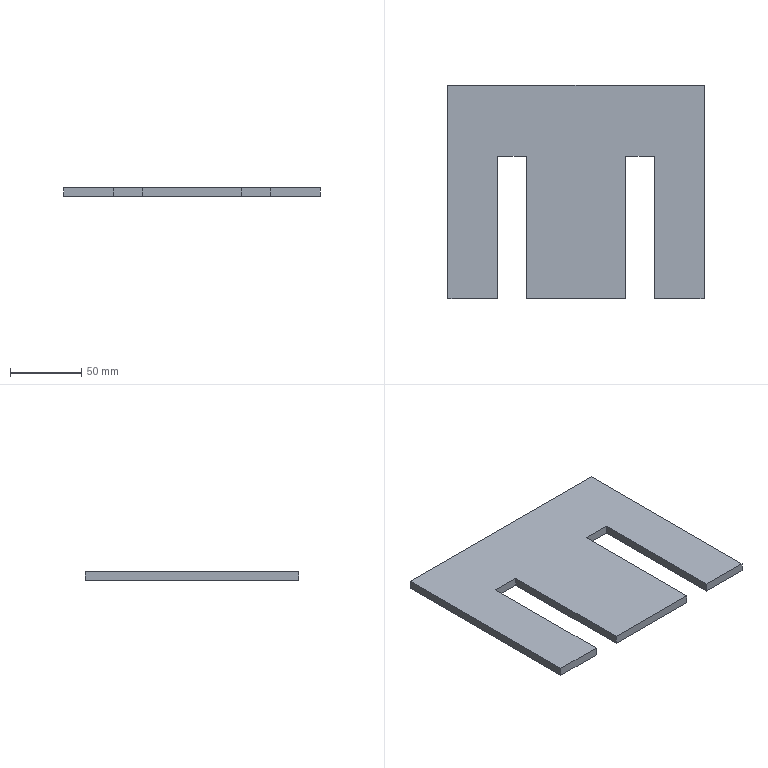Part | SolidWorks | features Extrusion 1, ICE 1, MirrorPattern 1 | 1 solid | 14 faces | box 180 x 150 x 6 mm | volume 138000 mm3 | plane 14
STEP:
#1=CARTESIAN_POINT('',(55.,-75.,0.));
#2=VERTEX_POINT('',#1);
#3=CARTESIAN_POINT('',(55.,-75.,6.));
#4=VERTEX_POINT('',#3);
#5=CARTESIAN_POINT('',(55.,-75.,-0.001));
#6=DIRECTION('',(0.,0.,1.));
#7=VECTOR('',#6,1000.);
#8=LINE('',#5,#7);
#9=EDGE_CURVE('',#2,#4,#8,.T.);
#10=ORIENTED_EDGE('',*,*,#9,.F.);
#11=CARTESIAN_POINT('',(90.,-75.,0.));
#12=VERTEX_POINT('',#11);
#13=CARTESIAN_POINT('',(-90.,-75.,0.));
#14=DIRECTION('',(1.,0.,0.));
#15=VECTOR('',#14,1000.);
#16=LINE('',#13,#15);
#17=EDGE_CURVE('',#2,#12,#16,.T.);
#18=ORIENTED_EDGE('',*,*,#17,.T.);
#19=CARTESIAN_POINT('',(90.,-75.,6.));
#20=VERTEX_POINT('',#19);
#21=CARTESIAN_POINT('',(90.,-75.,6.));
#22=DIRECTION('',(0.,0.,-1.));
#23=VECTOR('',#22,1000.);
#24=LINE('',#21,#23);
#25=EDGE_CURVE('',#20,#12,#24,.T.);
#26=ORIENTED_EDGE('',*,*,#25,.F.);
#27=CARTESIAN_POINT('',(-90.,-75.,6.));
#28=DIRECTION('',(1.,0.,0.));
#29=VECTOR('',#28,1000.);
#30=LINE('',#27,#29);
#31=EDGE_CURVE('',#4,#20,#30,.T.);
#32=ORIENTED_EDGE('',*,*,#31,.F.);
#33=EDGE_LOOP('',(#10,#18,#26,#32));
#34=FACE_OUTER_BOUND('',#33,.T.);
#35=CARTESIAN_POINT('',(-90.,-75.,6.));
#36=DIRECTION('',(0.,1.,0.));
#37=DIRECTION('',(0.,0.,1.));
#38=AXIS2_PLACEMENT_3D('',#35,#36,#37);
#39=PLANE('',#38);
#40=ADVANCED_FACE('',(#34),#39,.F.);
#41=CARTESIAN_POINT('',(35.,-75.,0.));
#42=VERTEX_POINT('',#41);
#43=CARTESIAN_POINT('',(35.,-75.,6.));
#44=VERTEX_POINT('',#43);
#45=CARTESIAN_POINT('',(35.,-75.,-0.001));
#46=DIRECTION('',(0.,0.,1.));
#47=VECTOR('',#46,1000.);
#48=LINE('',#45,#47);
#49=EDGE_CURVE('',#42,#44,#48,.T.);
#50=ORIENTED_EDGE('',*,*,#49,.T.);
#51=CARTESIAN_POINT('',(-35.,-75.,6.));
#52=VERTEX_POINT('',#51);
#53=CARTESIAN_POINT('',(-90.,-75.,6.));
#54=DIRECTION('',(1.,0.,0.));
#55=VECTOR('',#54,1000.);
#56=LINE('',#53,#55);
#57=EDGE_CURVE('',#52,#44,#56,.T.);
#58=ORIENTED_EDGE('',*,*,#57,.F.);
#59=CARTESIAN_POINT('',(-35.,-75.,0.));
#60=VERTEX_POINT('',#59);
#61=CARTESIAN_POINT('',(-35.,-75.,-0.001));
#62=DIRECTION('',(0.,0.,1.));
#63=VECTOR('',#62,1000.);
#64=LINE('',#61,#63);
#65=EDGE_CURVE('',#60,#52,#64,.T.);
#66=ORIENTED_EDGE('',*,*,#65,.F.);
#67=CARTESIAN_POINT('',(-90.,-75.,0.));
#68=DIRECTION('',(1.,0.,0.));
#69=VECTOR('',#68,1000.);
#70=LINE('',#67,#69);
#71=EDGE_CURVE('',#60,#42,#70,.T.);
#72=ORIENTED_EDGE('',*,*,#71,.T.);
#73=EDGE_LOOP('',(#50,#58,#66,#72));
#74=FACE_OUTER_BOUND('',#73,.T.);
#75=CARTESIAN_POINT('',(-90.,-75.,6.));
#76=DIRECTION('',(0.,1.,0.));
#77=DIRECTION('',(0.,0.,1.));
#78=AXIS2_PLACEMENT_3D('',#75,#76,#77);
#79=PLANE('',#78);
#80=ADVANCED_FACE('',(#74),#79,.F.);
#81=CARTESIAN_POINT('',(55.,25.,6.));
#82=VERTEX_POINT('',#81);
#83=CARTESIAN_POINT('',(55.,-75.,6.));
#84=DIRECTION('',(0.,-1.,0.));
#85=VECTOR('',#84,1000.);
#86=LINE('',#83,#85);
#87=EDGE_CURVE('',#82,#4,#86,.T.);
#88=ORIENTED_EDGE('',*,*,#87,.T.);
#89=ORIENTED_EDGE('',*,*,#31,.T.);
#90=CARTESIAN_POINT('',(90.,75.,6.));
#91=VERTEX_POINT('',#90);
#92=CARTESIAN_POINT('',(90.,-75.,6.));
#93=DIRECTION('',(0.,1.,0.));
#94=VECTOR('',#93,1000.);
#95=LINE('',#92,#94);
#96=EDGE_CURVE('',#20,#91,#95,.T.);
#97=ORIENTED_EDGE('',*,*,#96,.T.);
#98=CARTESIAN_POINT('',(-90.,75.,6.));
#99=VERTEX_POINT('',#98);
#100=CARTESIAN_POINT('',(-90.,75.,6.));
#101=DIRECTION('',(-1.,0.,0.));
#102=VECTOR('',#101,1000.);
#103=LINE('',#100,#102);
#104=EDGE_CURVE('',#91,#99,#103,.T.);
#105=ORIENTED_EDGE('',*,*,#104,.T.);
#106=CARTESIAN_POINT('',(-90.,-75.,6.));
#107=VERTEX_POINT('',#106);
#108=CARTESIAN_POINT('',(-90.,-75.,6.));
#109=DIRECTION('',(0.,-1.,0.));
#110=VECTOR('',#109,1000.);
#111=LINE('',#108,#110);
#112=EDGE_CURVE('',#99,#107,#111,.T.);
#113=ORIENTED_EDGE('',*,*,#112,.T.);
#114=CARTESIAN_POINT('',(-55.,-75.,6.));
#115=VERTEX_POINT('',#114);
#116=CARTESIAN_POINT('',(-90.,-75.,6.));
#117=DIRECTION('',(1.,0.,0.));
#118=VECTOR('',#117,1000.);
#119=LINE('',#116,#118);
#120=EDGE_CURVE('',#107,#115,#119,.T.);
#121=ORIENTED_EDGE('',*,*,#120,.T.);
#122=CARTESIAN_POINT('',(-55.,25.,6.));
#123=VERTEX_POINT('',#122);
#124=CARTESIAN_POINT('',(-55.,-75.,6.));
#125=DIRECTION('',(0.,-1.,0.));
#126=VECTOR('',#125,1000.);
#127=LINE('',#124,#126);
#128=EDGE_CURVE('',#123,#115,#127,.T.);
#129=ORIENTED_EDGE('',*,*,#128,.F.);
#130=CARTESIAN_POINT('',(-35.,25.,6.));
#131=VERTEX_POINT('',#130);
#132=CARTESIAN_POINT('',(-55.,25.,6.));
#133=DIRECTION('',(-1.,0.,0.));
#134=VECTOR('',#133,1000.);
#135=LINE('',#132,#134);
#136=EDGE_CURVE('',#131,#123,#135,.T.);
#137=ORIENTED_EDGE('',*,*,#136,.F.);
#138=CARTESIAN_POINT('',(-35.,-75.,6.));
#139=DIRECTION('',(0.,1.,0.));
#140=VECTOR('',#139,1000.);
#141=LINE('',#138,#140);
#142=EDGE_CURVE('',#52,#131,#141,.T.);
#143=ORIENTED_EDGE('',*,*,#142,.F.);
#144=ORIENTED_EDGE('',*,*,#57,.T.);
#145=CARTESIAN_POINT('',(35.,25.,6.));
#146=VERTEX_POINT('',#145);
#147=CARTESIAN_POINT('',(35.,-75.,6.));
#148=DIRECTION('',(0.,1.,0.));
#149=VECTOR('',#148,1000.);
#150=LINE('',#147,#149);
#151=EDGE_CURVE('',#44,#146,#150,.T.);
#152=ORIENTED_EDGE('',*,*,#151,.T.);
#153=CARTESIAN_POINT('',(55.,25.,6.));
#154=DIRECTION('',(1.,0.,0.));
#155=VECTOR('',#154,1000.);
#156=LINE('',#153,#155);
#157=EDGE_CURVE('',#146,#82,#156,.T.);
#158=ORIENTED_EDGE('',*,*,#157,.T.);
#159=EDGE_LOOP('',(#88,#89,#97,#105,#113,#121,#129,#137,#143,#144,#152,#158));
#160=FACE_OUTER_BOUND('',#159,.T.);
#161=CARTESIAN_POINT('',(0.,0.,6.));
#162=DIRECTION('',(0.,0.,-1.));
#163=DIRECTION('',(-1.,0.,0.));
#164=AXIS2_PLACEMENT_3D('',#161,#162,#163);
#165=PLANE('',#164);
#166=ADVANCED_FACE('',(#160),#165,.F.);
#167=ORIENTED_EDGE('',*,*,#17,.F.);
#168=CARTESIAN_POINT('',(55.,25.,0.));
#169=VERTEX_POINT('',#168);
#170=CARTESIAN_POINT('',(55.,-75.,0.));
#171=DIRECTION('',(0.,-1.,0.));
#172=VECTOR('',#171,1000.);
#173=LINE('',#170,#172);
#174=EDGE_CURVE('',#169,#2,#173,.T.);
#175=ORIENTED_EDGE('',*,*,#174,.F.);
#176=CARTESIAN_POINT('',(35.,25.,0.));
#177=VERTEX_POINT('',#176);
#178=CARTESIAN_POINT('',(55.,25.,0.));
#179=DIRECTION('',(1.,0.,0.));
#180=VECTOR('',#179,1000.);
#181=LINE('',#178,#180);
#182=EDGE_CURVE('',#177,#169,#181,.T.);
#183=ORIENTED_EDGE('',*,*,#182,.F.);
#184=CARTESIAN_POINT('',(35.,-75.,0.));
#185=DIRECTION('',(0.,1.,0.));
#186=VECTOR('',#185,1000.);
#187=LINE('',#184,#186);
#188=EDGE_CURVE('',#42,#177,#187,.T.);
#189=ORIENTED_EDGE('',*,*,#188,.F.);
#190=ORIENTED_EDGE('',*,*,#71,.F.);
#191=CARTESIAN_POINT('',(-35.,25.,0.));
#192=VERTEX_POINT('',#191);
#193=CARTESIAN_POINT('',(-35.,-75.,0.));
#194=DIRECTION('',(0.,1.,0.));
#195=VECTOR('',#194,1000.);
#196=LINE('',#193,#195);
#197=EDGE_CURVE('',#60,#192,#196,.T.);
#198=ORIENTED_EDGE('',*,*,#197,.T.);
#199=CARTESIAN_POINT('',(-55.,25.,0.));
#200=VERTEX_POINT('',#199);
#201=CARTESIAN_POINT('',(-55.,25.,0.));
#202=DIRECTION('',(-1.,0.,0.));
#203=VECTOR('',#202,1000.);
#204=LINE('',#201,#203);
#205=EDGE_CURVE('',#192,#200,#204,.T.);
#206=ORIENTED_EDGE('',*,*,#205,.T.);
#207=CARTESIAN_POINT('',(-55.,-75.,0.));
#208=VERTEX_POINT('',#207);
#209=CARTESIAN_POINT('',(-55.,-75.,0.));
#210=DIRECTION('',(0.,-1.,0.));
#211=VECTOR('',#210,1000.);
#212=LINE('',#209,#211);
#213=EDGE_CURVE('',#200,#208,#212,.T.);
#214=ORIENTED_EDGE('',*,*,#213,.T.);
#215=CARTESIAN_POINT('',(-90.,-75.,0.));
#216=VERTEX_POINT('',#215);
#217=CARTESIAN_POINT('',(-90.,-75.,0.));
#218=DIRECTION('',(1.,0.,0.));
#219=VECTOR('',#218,1000.);
#220=LINE('',#217,#219);
#221=EDGE_CURVE('',#216,#208,#220,.T.);
#222=ORIENTED_EDGE('',*,*,#221,.F.);
#223=CARTESIAN_POINT('',(-90.,75.,0.));
#224=VERTEX_POINT('',#223);
#225=CARTESIAN_POINT('',(-90.,-75.,0.));
#226=DIRECTION('',(0.,-1.,0.));
#227=VECTOR('',#226,1000.);
#228=LINE('',#225,#227);
#229=EDGE_CURVE('',#224,#216,#228,.T.);
#230=ORIENTED_EDGE('',*,*,#229,.F.);
#231=CARTESIAN_POINT('',(90.,75.,0.));
#232=VERTEX_POINT('',#231);
#233=CARTESIAN_POINT('',(-90.,75.,0.));
#234=DIRECTION('',(-1.,0.,0.));
#235=VECTOR('',#234,1000.);
#236=LINE('',#233,#235);
#237=EDGE_CURVE('',#232,#224,#236,.T.);
#238=ORIENTED_EDGE('',*,*,#237,.F.);
#239=CARTESIAN_POINT('',(90.,-75.,0.));
#240=DIRECTION('',(0.,1.,0.));
#241=VECTOR('',#240,1000.);
#242=LINE('',#239,#241);
#243=EDGE_CURVE('',#12,#232,#242,.T.);
#244=ORIENTED_EDGE('',*,*,#243,.F.);
#245=EDGE_LOOP('',(#167,#175,#183,#189,#190,#198,#206,#214,#222,#230,#238,#244));
#246=FACE_OUTER_BOUND('',#245,.T.);
#247=CARTESIAN_POINT('',(0.,0.,0.));
#248=DIRECTION('',(0.,0.,-1.));
#249=DIRECTION('',(-1.,0.,0.));
#250=AXIS2_PLACEMENT_3D('',#247,#248,#249);
#251=PLANE('',#250);
#252=ADVANCED_FACE('',(#246),#251,.T.);
#253=ORIENTED_EDGE('',*,*,#221,.T.);
#254=CARTESIAN_POINT('',(-55.,-75.,-0.001));
#255=DIRECTION('',(0.,0.,1.));
#256=VECTOR('',#255,1000.);
#257=LINE('',#254,#256);
#258=EDGE_CURVE('',#208,#115,#257,.T.);
#259=ORIENTED_EDGE('',*,*,#258,.T.);
#260=ORIENTED_EDGE('',*,*,#120,.F.);
#261=CARTESIAN_POINT('',(-90.,-75.,6.));
#262=DIRECTION('',(0.,0.,-1.));
#263=VECTOR('',#262,1000.);
#264=LINE('',#261,#263);
#265=EDGE_CURVE('',#107,#216,#264,.T.);
#266=ORIENTED_EDGE('',*,*,#265,.T.);
#267=EDGE_LOOP('',(#253,#259,#260,#266));
#268=FACE_OUTER_BOUND('',#267,.T.);
#269=CARTESIAN_POINT('',(-90.,-75.,6.));
#270=DIRECTION('',(0.,1.,0.));
#271=DIRECTION('',(0.,0.,1.));
#272=AXIS2_PLACEMENT_3D('',#269,#270,#271);
#273=PLANE('',#272);
#274=ADVANCED_FACE('',(#268),#273,.F.);
#275=ORIENTED_EDGE('',*,*,#243,.T.);
#276=CARTESIAN_POINT('',(90.,75.,6.));
#277=DIRECTION('',(0.,0.,-1.));
#278=VECTOR('',#277,1000.);
#279=LINE('',#276,#278);
#280=EDGE_CURVE('',#91,#232,#279,.T.);
#281=ORIENTED_EDGE('',*,*,#280,.F.);
#282=ORIENTED_EDGE('',*,*,#96,.F.);
#283=ORIENTED_EDGE('',*,*,#25,.T.);
#284=EDGE_LOOP('',(#275,#281,#282,#283));
#285=FACE_OUTER_BOUND('',#284,.T.);
#286=CARTESIAN_POINT('',(90.,-75.,6.));
#287=DIRECTION('',(-1.,0.,0.));
#288=DIRECTION('',(0.,0.,1.));
#289=AXIS2_PLACEMENT_3D('',#286,#287,#288);
#290=PLANE('',#289);
#291=ADVANCED_FACE('',(#285),#290,.F.);
#292=ORIENTED_EDGE('',*,*,#237,.T.);
#293=CARTESIAN_POINT('',(-90.,75.,6.));
#294=DIRECTION('',(0.,0.,-1.));
#295=VECTOR('',#294,1000.);
#296=LINE('',#293,#295);
#297=EDGE_CURVE('',#99,#224,#296,.T.);
#298=ORIENTED_EDGE('',*,*,#297,.F.);
#299=ORIENTED_EDGE('',*,*,#104,.F.);
#300=ORIENTED_EDGE('',*,*,#280,.T.);
#301=EDGE_LOOP('',(#292,#298,#299,#300));
#302=FACE_OUTER_BOUND('',#301,.T.);
#303=CARTESIAN_POINT('',(-90.,75.,6.));
#304=DIRECTION('',(0.,-1.,0.));
#305=DIRECTION('',(0.,0.,-1.));
#306=AXIS2_PLACEMENT_3D('',#303,#304,#305);
#307=PLANE('',#306);
#308=ADVANCED_FACE('',(#302),#307,.F.);
#309=ORIENTED_EDGE('',*,*,#229,.T.);
#310=ORIENTED_EDGE('',*,*,#265,.F.);
#311=ORIENTED_EDGE('',*,*,#112,.F.);
#312=ORIENTED_EDGE('',*,*,#297,.T.);
#313=EDGE_LOOP('',(#309,#310,#311,#312));
#314=FACE_OUTER_BOUND('',#313,.T.);
#315=CARTESIAN_POINT('',(-90.,-75.,6.));
#316=DIRECTION('',(1.,0.,0.));
#317=DIRECTION('',(0.,0.,-1.));
#318=AXIS2_PLACEMENT_3D('',#315,#316,#317);
#319=PLANE('',#318);
#320=ADVANCED_FACE('',(#314),#319,.F.);
#321=CARTESIAN_POINT('',(-55.,25.,-0.001));
#322=DIRECTION('',(0.,0.,1.));
#323=VECTOR('',#322,1000.);
#324=LINE('',#321,#323);
#325=EDGE_CURVE('',#200,#123,#324,.T.);
#326=ORIENTED_EDGE('',*,*,#325,.T.);
#327=ORIENTED_EDGE('',*,*,#128,.T.);
#328=ORIENTED_EDGE('',*,*,#258,.F.);
#329=ORIENTED_EDGE('',*,*,#213,.F.);
#330=EDGE_LOOP('',(#326,#327,#328,#329));
#331=FACE_OUTER_BOUND('',#330,.T.);
#332=CARTESIAN_POINT('',(-55.,-75.,-0.001));
#333=DIRECTION('',(-1.,0.,0.));
#334=DIRECTION('',(0.,0.,1.));
#335=AXIS2_PLACEMENT_3D('',#332,#333,#334);
#336=PLANE('',#335);
#337=ADVANCED_FACE('',(#331),#336,.F.);
#338=CARTESIAN_POINT('',(-35.,25.,-0.001));
#339=DIRECTION('',(0.,0.,1.));
#340=VECTOR('',#339,1000.);
#341=LINE('',#338,#340);
#342=EDGE_CURVE('',#192,#131,#341,.T.);
#343=ORIENTED_EDGE('',*,*,#342,.T.);
#344=ORIENTED_EDGE('',*,*,#136,.T.);
#345=ORIENTED_EDGE('',*,*,#325,.F.);
#346=ORIENTED_EDGE('',*,*,#205,.F.);
#347=EDGE_LOOP('',(#343,#344,#345,#346));
#348=FACE_OUTER_BOUND('',#347,.T.);
#349=CARTESIAN_POINT('',(-55.,25.,-0.001));
#350=DIRECTION('',(0.,1.,0.));
#351=DIRECTION('',(0.,0.,1.));
#352=AXIS2_PLACEMENT_3D('',#349,#350,#351);
#353=PLANE('',#352);
#354=ADVANCED_FACE('',(#348),#353,.F.);
#355=ORIENTED_EDGE('',*,*,#65,.T.);
#356=ORIENTED_EDGE('',*,*,#142,.T.);
#357=ORIENTED_EDGE('',*,*,#342,.F.);
#358=ORIENTED_EDGE('',*,*,#197,.F.);
#359=EDGE_LOOP('',(#355,#356,#357,#358));
#360=FACE_OUTER_BOUND('',#359,.T.);
#361=CARTESIAN_POINT('',(-35.,-75.,-0.001));
#362=DIRECTION('',(1.,0.,0.));
#363=DIRECTION('',(0.,0.,-1.));
#364=AXIS2_PLACEMENT_3D('',#361,#362,#363);
#365=PLANE('',#364);
#366=ADVANCED_FACE('',(#360),#365,.F.);
#367=ORIENTED_EDGE('',*,*,#174,.T.);
#368=ORIENTED_EDGE('',*,*,#9,.T.);
#369=ORIENTED_EDGE('',*,*,#87,.F.);
#370=CARTESIAN_POINT('',(55.,25.,-0.001));
#371=DIRECTION('',(0.,0.,1.));
#372=VECTOR('',#371,1000.);
#373=LINE('',#370,#372);
#374=EDGE_CURVE('',#169,#82,#373,.T.);
#375=ORIENTED_EDGE('',*,*,#374,.F.);
#376=EDGE_LOOP('',(#367,#368,#369,#375));
#377=FACE_OUTER_BOUND('',#376,.T.);
#378=CARTESIAN_POINT('',(55.,-75.,-0.001));
#379=DIRECTION('',(-1.,0.,0.));
#380=DIRECTION('',(0.,0.,1.));
#381=AXIS2_PLACEMENT_3D('',#378,#379,#380);
#382=PLANE('',#381);
#383=ADVANCED_FACE('',(#377),#382,.T.);
#384=ORIENTED_EDGE('',*,*,#188,.T.);
#385=CARTESIAN_POINT('',(35.,25.,-0.001));
#386=DIRECTION('',(0.,0.,1.));
#387=VECTOR('',#386,1000.);
#388=LINE('',#385,#387);
#389=EDGE_CURVE('',#177,#146,#388,.T.);
#390=ORIENTED_EDGE('',*,*,#389,.T.);
#391=ORIENTED_EDGE('',*,*,#151,.F.);
#392=ORIENTED_EDGE('',*,*,#49,.F.);
#393=EDGE_LOOP('',(#384,#390,#391,#392));
#394=FACE_OUTER_BOUND('',#393,.T.);
#395=CARTESIAN_POINT('',(35.,-75.,-0.001));
#396=DIRECTION('',(1.,0.,0.));
#397=DIRECTION('',(0.,0.,-1.));
#398=AXIS2_PLACEMENT_3D('',#395,#396,#397);
#399=PLANE('',#398);
#400=ADVANCED_FACE('',(#394),#399,.T.);
#401=ORIENTED_EDGE('',*,*,#182,.T.);
#402=ORIENTED_EDGE('',*,*,#374,.T.);
#403=ORIENTED_EDGE('',*,*,#157,.F.);
#404=ORIENTED_EDGE('',*,*,#389,.F.);
#405=EDGE_LOOP('',(#401,#402,#403,#404));
#406=FACE_OUTER_BOUND('',#405,.T.);
#407=CARTESIAN_POINT('',(55.,25.,-0.001));
#408=DIRECTION('',(0.,-1.,0.));
#409=DIRECTION('',(0.,0.,-1.));
#410=AXIS2_PLACEMENT_3D('',#407,#408,#409);
#411=PLANE('',#410);
#412=ADVANCED_FACE('',(#406),#411,.T.);
#413=CLOSED_SHELL('',(#40,#80,#166,#252,#274,#291,#308,#320,#337,#354,#366,#383,#400,#412));
#414=MANIFOLD_SOLID_BREP('',#413);
#415=CARTESIAN_POINT('',(0.,0.,0.));
#416=DIRECTION('',(0.,0.,1.));
#417=DIRECTION('',(1.,0.,0.));
#418=AXIS2_PLACEMENT_3D('',#415,#416,#417);
#419=(LENGTH_UNIT()NAMED_UNIT(*)SI_UNIT(.MILLI.,.METRE.));
#420=UNCERTAINTY_MEASURE_WITH_UNIT(LENGTH_MEASURE(0.00001),#419,'','');
#421=(NAMED_UNIT(*)PLANE_ANGLE_UNIT()SI_UNIT($,.RADIAN.));
#422=(NAMED_UNIT(*)SI_UNIT($,.STERADIAN.)SOLID_ANGLE_UNIT());
#423=(GEOMETRIC_REPRESENTATION_CONTEXT(3)GLOBAL_UNCERTAINTY_ASSIGNED_CONTEXT((#420))GLOBAL_UNIT_ASSIGNED_CONTEXT((#419,#421,#422))REPRESENTATION_CONTEXT('',''));
#424=ADVANCED_BREP_SHAPE_REPRESENTATION('',(#414,#418),#423);